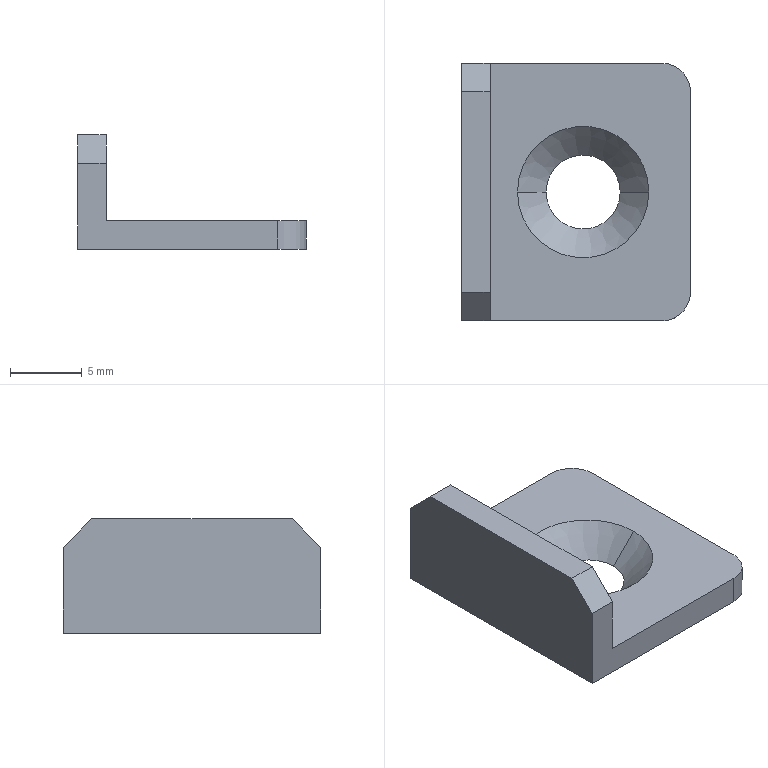Part | SolidWorks | features BaseBody 1 | 1 solid | 14 faces | box 16 x 18 x 8 mm | volume 697.494 mm3 | plane 10 | cone 2 | cylinder 2 | commonest cylinder face diameters 4 x2
STEP:
#1=CARTESIAN_POINT('',(-8.,-9.,4.));
#2=VERTEX_POINT('',#1);
#3=CARTESIAN_POINT('',(-8.,-7.,6.));
#4=VERTEX_POINT('',#3);
#5=CARTESIAN_POINT('',(-8.,-12.,1.));
#6=DIRECTION('',(0.,0.7071,0.7071));
#7=VECTOR('',#6,1000.);
#8=LINE('',#5,#7);
#9=EDGE_CURVE('',#2,#4,#8,.T.);
#10=ORIENTED_EDGE('',*,*,#9,.F.);
#11=CARTESIAN_POINT('',(-6.,-9.,4.));
#12=VERTEX_POINT('',#11);
#13=CARTESIAN_POINT('',(8.,-9.,4.));
#14=DIRECTION('',(-1.,0.,0.));
#15=VECTOR('',#14,1000.);
#16=LINE('',#13,#15);
#17=EDGE_CURVE('',#12,#2,#16,.T.);
#18=ORIENTED_EDGE('',*,*,#17,.F.);
#19=CARTESIAN_POINT('',(-6.,-7.,6.));
#20=VERTEX_POINT('',#19);
#21=CARTESIAN_POINT('',(-6.,-7.,6.));
#22=DIRECTION('',(0.,-0.7071,-0.7071));
#23=VECTOR('',#22,1000.);
#24=LINE('',#21,#23);
#25=EDGE_CURVE('',#20,#12,#24,.T.);
#26=ORIENTED_EDGE('',*,*,#25,.F.);
#27=CARTESIAN_POINT('',(0.,-7.,6.));
#28=DIRECTION('',(1.,0.,0.));
#29=VECTOR('',#28,1000.);
#30=LINE('',#27,#29);
#31=EDGE_CURVE('',#4,#20,#30,.T.);
#32=ORIENTED_EDGE('',*,*,#31,.F.);
#33=EDGE_LOOP('',(#10,#18,#26,#32));
#34=FACE_OUTER_BOUND('',#33,.T.);
#35=CARTESIAN_POINT('',(0.,-7.,6.));
#36=DIRECTION('',(0.,0.7071,-0.7071));
#37=DIRECTION('',(-1.,0.,0.));
#38=AXIS2_PLACEMENT_3D('',#35,#36,#37);
#39=PLANE('',#38);
#40=ADVANCED_FACE('',(#34),#39,.F.);
#41=CARTESIAN_POINT('',(-6.,9.,4.));
#42=VERTEX_POINT('',#41);
#43=CARTESIAN_POINT('',(-6.,7.,6.));
#44=VERTEX_POINT('',#43);
#45=CARTESIAN_POINT('',(-6.,7.,6.));
#46=DIRECTION('',(0.,-0.7071,0.7071));
#47=VECTOR('',#46,1000.);
#48=LINE('',#45,#47);
#49=EDGE_CURVE('',#42,#44,#48,.T.);
#50=ORIENTED_EDGE('',*,*,#49,.F.);
#51=CARTESIAN_POINT('',(-8.,9.,4.));
#52=VERTEX_POINT('',#51);
#53=CARTESIAN_POINT('',(8.,9.,4.));
#54=DIRECTION('',(1.,0.,0.));
#55=VECTOR('',#54,1000.);
#56=LINE('',#53,#55);
#57=EDGE_CURVE('',#52,#42,#56,.T.);
#58=ORIENTED_EDGE('',*,*,#57,.F.);
#59=CARTESIAN_POINT('',(-8.,7.,6.));
#60=VERTEX_POINT('',#59);
#61=CARTESIAN_POINT('',(-8.,3.,10.));
#62=DIRECTION('',(0.,0.7071,-0.7071));
#63=VECTOR('',#62,1000.);
#64=LINE('',#61,#63);
#65=EDGE_CURVE('',#60,#52,#64,.T.);
#66=ORIENTED_EDGE('',*,*,#65,.F.);
#67=CARTESIAN_POINT('',(0.,7.,6.));
#68=DIRECTION('',(-1.,0.,0.));
#69=VECTOR('',#68,1000.);
#70=LINE('',#67,#69);
#71=EDGE_CURVE('',#44,#60,#70,.T.);
#72=ORIENTED_EDGE('',*,*,#71,.F.);
#73=EDGE_LOOP('',(#50,#58,#66,#72));
#74=FACE_OUTER_BOUND('',#73,.T.);
#75=CARTESIAN_POINT('',(0.,7.,6.));
#76=DIRECTION('',(0.,-0.7071,-0.7071));
#77=DIRECTION('',(0.,0.7071,-0.7071));
#78=AXIS2_PLACEMENT_3D('',#75,#76,#77);
#79=PLANE('',#78);
#80=ADVANCED_FACE('',(#74),#79,.F.);
#81=CARTESIAN_POINT('',(-6.,9.,6.));
#82=DIRECTION('',(0.,1.,0.));
#83=VECTOR('',#82,1000.);
#84=LINE('',#81,#83);
#85=EDGE_CURVE('',#20,#44,#84,.T.);
#86=ORIENTED_EDGE('',*,*,#85,.T.);
#87=ORIENTED_EDGE('',*,*,#71,.T.);
#88=CARTESIAN_POINT('',(-8.,9.,6.));
#89=DIRECTION('',(0.,-1.,0.));
#90=VECTOR('',#89,1000.);
#91=LINE('',#88,#90);
#92=EDGE_CURVE('',#60,#4,#91,.T.);
#93=ORIENTED_EDGE('',*,*,#92,.T.);
#94=ORIENTED_EDGE('',*,*,#31,.T.);
#95=EDGE_LOOP('',(#86,#87,#93,#94));
#96=FACE_OUTER_BOUND('',#95,.T.);
#97=CARTESIAN_POINT('',(0.,0.,6.));
#98=DIRECTION('',(0.,0.,1.));
#99=DIRECTION('',(1.,0.,0.));
#100=AXIS2_PLACEMENT_3D('',#97,#98,#99);
#101=PLANE('',#100);
#102=ADVANCED_FACE('',(#96),#101,.T.);
#103=CARTESIAN_POINT('',(-6.,9.,0.));
#104=VERTEX_POINT('',#103);
#105=CARTESIAN_POINT('',(-6.,9.,6.));
#106=DIRECTION('',(0.,0.,-1.));
#107=VECTOR('',#106,1000.);
#108=LINE('',#105,#107);
#109=EDGE_CURVE('',#42,#104,#108,.T.);
#110=ORIENTED_EDGE('',*,*,#109,.F.);
#111=ORIENTED_EDGE('',*,*,#49,.T.);
#112=ORIENTED_EDGE('',*,*,#85,.F.);
#113=ORIENTED_EDGE('',*,*,#25,.T.);
#114=CARTESIAN_POINT('',(-6.,-9.,0.));
#115=VERTEX_POINT('',#114);
#116=CARTESIAN_POINT('',(-6.,-9.,6.));
#117=DIRECTION('',(0.,0.,-1.));
#118=VECTOR('',#117,1000.);
#119=LINE('',#116,#118);
#120=EDGE_CURVE('',#12,#115,#119,.T.);
#121=ORIENTED_EDGE('',*,*,#120,.T.);
#122=CARTESIAN_POINT('',(-6.,9.,0.));
#123=DIRECTION('',(0.,1.,0.));
#124=VECTOR('',#123,1000.);
#125=LINE('',#122,#124);
#126=EDGE_CURVE('',#115,#104,#125,.T.);
#127=ORIENTED_EDGE('',*,*,#126,.T.);
#128=EDGE_LOOP('',(#110,#111,#112,#113,#121,#127));
#129=FACE_OUTER_BOUND('',#128,.T.);
#130=CARTESIAN_POINT('',(-6.,9.,6.));
#131=DIRECTION('',(-1.,0.,0.));
#132=DIRECTION('',(0.,1.,0.));
#133=AXIS2_PLACEMENT_3D('',#130,#131,#132);
#134=PLANE('',#133);
#135=ADVANCED_FACE('',(#129),#134,.F.);
#136=CARTESIAN_POINT('',(-2.09,0.,-2.));
#137=VERTEX_POINT('',#136);
#138=CARTESIAN_POINT('',(-4.09,0.,0.));
#139=VERTEX_POINT('',#138);
#140=CARTESIAN_POINT('',(-4.09,0.,0.));
#141=DIRECTION('',(-0.7071,0.,0.7071));
#142=VECTOR('',#141,1000.);
#143=LINE('',#140,#142);
#144=EDGE_CURVE('',#137,#139,#143,.T.);
#145=ORIENTED_EDGE('',*,*,#144,.F.);
#146=CARTESIAN_POINT('',(3.09,0.,-2.));
#147=VERTEX_POINT('',#146);
#148=CARTESIAN_POINT('',(0.5,0.,-2.));
#149=DIRECTION('',(0.,0.,1.));
#150=DIRECTION('',(1.,0.,0.));
#151=AXIS2_PLACEMENT_3D('',#148,#149,#150);
#152=CIRCLE('',#151,2.59);
#153=EDGE_CURVE('',#147,#137,#152,.T.);
#154=ORIENTED_EDGE('',*,*,#153,.F.);
#155=CARTESIAN_POINT('',(5.09,0.,0.));
#156=VERTEX_POINT('',#155);
#157=CARTESIAN_POINT('',(5.09,0.,0.));
#158=DIRECTION('',(0.7071,0.,0.7071));
#159=VECTOR('',#158,1000.);
#160=LINE('',#157,#159);
#161=EDGE_CURVE('',#147,#156,#160,.T.);
#162=ORIENTED_EDGE('',*,*,#161,.T.);
#163=CARTESIAN_POINT('',(0.5,0.,0.));
#164=DIRECTION('',(0.,0.,1.));
#165=DIRECTION('',(1.,0.,0.));
#166=AXIS2_PLACEMENT_3D('',#163,#164,#165);
#167=CIRCLE('',#166,4.59);
#168=EDGE_CURVE('',#156,#139,#167,.T.);
#169=ORIENTED_EDGE('',*,*,#168,.T.);
#170=EDGE_LOOP('',(#145,#154,#162,#169));
#171=FACE_OUTER_BOUND('',#170,.T.);
#172=CARTESIAN_POINT('',(0.5,0.,0.));
#173=DIRECTION('',(0.,0.,1.));
#174=DIRECTION('',(1.,0.,0.));
#175=AXIS2_PLACEMENT_3D('',#172,#173,#174);
#176=CONICAL_SURFACE('',#175,4.59,0.7854);
#177=ADVANCED_FACE('',(#171),#176,.F.);
#178=CARTESIAN_POINT('',(8.,-7.,-2.));
#179=VERTEX_POINT('',#178);
#180=CARTESIAN_POINT('',(6.,-9.,-2.));
#181=VERTEX_POINT('',#180);
#182=CARTESIAN_POINT('',(6.,-7.,-2.));
#183=DIRECTION('',(0.,0.,-1.));
#184=DIRECTION('',(1.,0.,0.));
#185=AXIS2_PLACEMENT_3D('',#182,#183,#184);
#186=CIRCLE('',#185,2.);
#187=EDGE_CURVE('',#179,#181,#186,.T.);
#188=ORIENTED_EDGE('',*,*,#187,.F.);
#189=CARTESIAN_POINT('',(8.,-7.,0.));
#190=VERTEX_POINT('',#189);
#191=CARTESIAN_POINT('',(8.,-7.,-2.));
#192=DIRECTION('',(0.,0.,-1.));
#193=VECTOR('',#192,1000.);
#194=LINE('',#191,#193);
#195=EDGE_CURVE('',#190,#179,#194,.T.);
#196=ORIENTED_EDGE('',*,*,#195,.F.);
#197=CARTESIAN_POINT('',(6.,-9.,0.));
#198=VERTEX_POINT('',#197);
#199=CARTESIAN_POINT('',(6.,-7.,0.));
#200=DIRECTION('',(0.,0.,1.));
#201=DIRECTION('',(1.,0.,0.));
#202=AXIS2_PLACEMENT_3D('',#199,#200,#201);
#203=CIRCLE('',#202,2.);
#204=EDGE_CURVE('',#198,#190,#203,.T.);
#205=ORIENTED_EDGE('',*,*,#204,.F.);
#206=CARTESIAN_POINT('',(6.,-9.,-2.));
#207=DIRECTION('',(0.,0.,1.));
#208=VECTOR('',#207,1000.);
#209=LINE('',#206,#208);
#210=EDGE_CURVE('',#181,#198,#209,.T.);
#211=ORIENTED_EDGE('',*,*,#210,.F.);
#212=EDGE_LOOP('',(#188,#196,#205,#211));
#213=FACE_OUTER_BOUND('',#212,.T.);
#214=CARTESIAN_POINT('',(6.,-7.,-2.));
#215=DIRECTION('',(0.,0.,1.));
#216=DIRECTION('',(1.,0.,0.));
#217=AXIS2_PLACEMENT_3D('',#214,#215,#216);
#218=CYLINDRICAL_SURFACE('',#217,2.);
#219=ADVANCED_FACE('',(#213),#218,.T.);
#220=CARTESIAN_POINT('',(6.,9.,-2.));
#221=VERTEX_POINT('',#220);
#222=CARTESIAN_POINT('',(8.,7.,-2.));
#223=VERTEX_POINT('',#222);
#224=CARTESIAN_POINT('',(6.,7.,-2.));
#225=DIRECTION('',(0.,0.,-1.));
#226=DIRECTION('',(1.,0.,0.));
#227=AXIS2_PLACEMENT_3D('',#224,#225,#226);
#228=CIRCLE('',#227,2.);
#229=EDGE_CURVE('',#221,#223,#228,.T.);
#230=ORIENTED_EDGE('',*,*,#229,.F.);
#231=CARTESIAN_POINT('',(6.,9.,0.));
#232=VERTEX_POINT('',#231);
#233=CARTESIAN_POINT('',(6.,9.,-2.));
#234=DIRECTION('',(0.,0.,-1.));
#235=VECTOR('',#234,1000.);
#236=LINE('',#233,#235);
#237=EDGE_CURVE('',#232,#221,#236,.T.);
#238=ORIENTED_EDGE('',*,*,#237,.F.);
#239=CARTESIAN_POINT('',(8.,7.,0.));
#240=VERTEX_POINT('',#239);
#241=CARTESIAN_POINT('',(6.,7.,0.));
#242=DIRECTION('',(0.,0.,1.));
#243=DIRECTION('',(1.,0.,0.));
#244=AXIS2_PLACEMENT_3D('',#241,#242,#243);
#245=CIRCLE('',#244,2.);
#246=EDGE_CURVE('',#240,#232,#245,.T.);
#247=ORIENTED_EDGE('',*,*,#246,.F.);
#248=CARTESIAN_POINT('',(8.,7.,-2.));
#249=DIRECTION('',(0.,0.,1.));
#250=VECTOR('',#249,1000.);
#251=LINE('',#248,#250);
#252=EDGE_CURVE('',#223,#240,#251,.T.);
#253=ORIENTED_EDGE('',*,*,#252,.F.);
#254=EDGE_LOOP('',(#230,#238,#247,#253));
#255=FACE_OUTER_BOUND('',#254,.T.);
#256=CARTESIAN_POINT('',(6.,7.,-2.));
#257=DIRECTION('',(0.,0.,1.));
#258=DIRECTION('',(1.,0.,0.));
#259=AXIS2_PLACEMENT_3D('',#256,#257,#258);
#260=CYLINDRICAL_SURFACE('',#259,2.);
#261=ADVANCED_FACE('',(#255),#260,.T.);
#262=ORIENTED_EDGE('',*,*,#168,.F.);
#263=CARTESIAN_POINT('',(0.5,0.,0.));
#264=DIRECTION('',(0.,0.,1.));
#265=DIRECTION('',(1.,0.,0.));
#266=AXIS2_PLACEMENT_3D('',#263,#264,#265);
#267=CIRCLE('',#266,4.59);
#268=EDGE_CURVE('',#139,#156,#267,.T.);
#269=ORIENTED_EDGE('',*,*,#268,.F.);
#270=EDGE_LOOP('',(#262,#269));
#271=FACE_BOUND('',#270,.T.);
#272=ORIENTED_EDGE('',*,*,#126,.F.);
#273=CARTESIAN_POINT('',(8.,-9.,0.));
#274=DIRECTION('',(1.,0.,0.));
#275=VECTOR('',#274,1000.);
#276=LINE('',#273,#275);
#277=EDGE_CURVE('',#115,#198,#276,.T.);
#278=ORIENTED_EDGE('',*,*,#277,.T.);
#279=ORIENTED_EDGE('',*,*,#204,.T.);
#280=CARTESIAN_POINT('',(8.,-9.,0.));
#281=DIRECTION('',(0.,1.,0.));
#282=VECTOR('',#281,1000.);
#283=LINE('',#280,#282);
#284=EDGE_CURVE('',#190,#240,#283,.T.);
#285=ORIENTED_EDGE('',*,*,#284,.T.);
#286=ORIENTED_EDGE('',*,*,#246,.T.);
#287=CARTESIAN_POINT('',(8.,9.,0.));
#288=DIRECTION('',(-1.,0.,0.));
#289=VECTOR('',#288,1000.);
#290=LINE('',#287,#289);
#291=EDGE_CURVE('',#232,#104,#290,.T.);
#292=ORIENTED_EDGE('',*,*,#291,.T.);
#293=EDGE_LOOP('',(#272,#278,#279,#285,#286,#292));
#294=FACE_OUTER_BOUND('',#293,.T.);
#295=CARTESIAN_POINT('',(0.,0.,0.));
#296=DIRECTION('',(0.,0.,1.));
#297=DIRECTION('',(1.,0.,0.));
#298=AXIS2_PLACEMENT_3D('',#295,#296,#297);
#299=PLANE('',#298);
#300=ADVANCED_FACE('',(#271,#294),#299,.T.);
#301=ORIENTED_EDGE('',*,*,#153,.T.);
#302=CARTESIAN_POINT('',(0.5,0.,-2.));
#303=DIRECTION('',(0.,0.,1.));
#304=DIRECTION('',(1.,0.,0.));
#305=AXIS2_PLACEMENT_3D('',#302,#303,#304);
#306=CIRCLE('',#305,2.59);
#307=EDGE_CURVE('',#137,#147,#306,.T.);
#308=ORIENTED_EDGE('',*,*,#307,.T.);
#309=EDGE_LOOP('',(#301,#308));
#310=FACE_BOUND('',#309,.T.);
#311=CARTESIAN_POINT('',(-8.,9.,-2.));
#312=VERTEX_POINT('',#311);
#313=CARTESIAN_POINT('',(8.,9.,-2.));
#314=DIRECTION('',(-1.,0.,0.));
#315=VECTOR('',#314,1000.);
#316=LINE('',#313,#315);
#317=EDGE_CURVE('',#221,#312,#316,.T.);
#318=ORIENTED_EDGE('',*,*,#317,.F.);
#319=ORIENTED_EDGE('',*,*,#229,.T.);
#320=CARTESIAN_POINT('',(8.,-9.,-2.));
#321=DIRECTION('',(0.,1.,0.));
#322=VECTOR('',#321,1000.);
#323=LINE('',#320,#322);
#324=EDGE_CURVE('',#179,#223,#323,.T.);
#325=ORIENTED_EDGE('',*,*,#324,.F.);
#326=ORIENTED_EDGE('',*,*,#187,.T.);
#327=CARTESIAN_POINT('',(-8.,-9.,-2.));
#328=VERTEX_POINT('',#327);
#329=CARTESIAN_POINT('',(8.,-9.,-2.));
#330=DIRECTION('',(1.,0.,0.));
#331=VECTOR('',#330,1000.);
#332=LINE('',#329,#331);
#333=EDGE_CURVE('',#328,#181,#332,.T.);
#334=ORIENTED_EDGE('',*,*,#333,.F.);
#335=CARTESIAN_POINT('',(-8.,-9.,-2.));
#336=DIRECTION('',(0.,-1.,0.));
#337=VECTOR('',#336,1000.);
#338=LINE('',#335,#337);
#339=EDGE_CURVE('',#312,#328,#338,.T.);
#340=ORIENTED_EDGE('',*,*,#339,.F.);
#341=EDGE_LOOP('',(#318,#319,#325,#326,#334,#340));
#342=FACE_OUTER_BOUND('',#341,.T.);
#343=CARTESIAN_POINT('',(0.,0.,-2.));
#344=DIRECTION('',(0.,0.,1.));
#345=DIRECTION('',(1.,0.,0.));
#346=AXIS2_PLACEMENT_3D('',#343,#344,#345);
#347=PLANE('',#346);
#348=ADVANCED_FACE('',(#310,#342),#347,.F.);
#349=ORIENTED_EDGE('',*,*,#120,.F.);
#350=ORIENTED_EDGE('',*,*,#17,.T.);
#351=CARTESIAN_POINT('',(-8.,-9.,-2.));
#352=DIRECTION('',(0.,0.,1.));
#353=VECTOR('',#352,1000.);
#354=LINE('',#351,#353);
#355=EDGE_CURVE('',#328,#2,#354,.T.);
#356=ORIENTED_EDGE('',*,*,#355,.F.);
#357=ORIENTED_EDGE('',*,*,#333,.T.);
#358=ORIENTED_EDGE('',*,*,#210,.T.);
#359=ORIENTED_EDGE('',*,*,#277,.F.);
#360=EDGE_LOOP('',(#349,#350,#356,#357,#358,#359));
#361=FACE_OUTER_BOUND('',#360,.T.);
#362=CARTESIAN_POINT('',(8.,-9.,-2.));
#363=DIRECTION('',(0.,-1.,0.));
#364=DIRECTION('',(0.,0.,-1.));
#365=AXIS2_PLACEMENT_3D('',#362,#363,#364);
#366=PLANE('',#365);
#367=ADVANCED_FACE('',(#361),#366,.T.);
#368=ORIENTED_EDGE('',*,*,#324,.T.);
#369=ORIENTED_EDGE('',*,*,#252,.T.);
#370=ORIENTED_EDGE('',*,*,#284,.F.);
#371=ORIENTED_EDGE('',*,*,#195,.T.);
#372=EDGE_LOOP('',(#368,#369,#370,#371));
#373=FACE_OUTER_BOUND('',#372,.T.);
#374=CARTESIAN_POINT('',(8.,-9.,-2.));
#375=DIRECTION('',(1.,0.,0.));
#376=DIRECTION('',(0.,1.,0.));
#377=AXIS2_PLACEMENT_3D('',#374,#375,#376);
#378=PLANE('',#377);
#379=ADVANCED_FACE('',(#373),#378,.T.);
#380=CARTESIAN_POINT('',(-8.,9.,-2.));
#381=DIRECTION('',(0.,0.,1.));
#382=VECTOR('',#381,1000.);
#383=LINE('',#380,#382);
#384=EDGE_CURVE('',#312,#52,#383,.T.);
#385=ORIENTED_EDGE('',*,*,#384,.T.);
#386=ORIENTED_EDGE('',*,*,#57,.T.);
#387=ORIENTED_EDGE('',*,*,#109,.T.);
#388=ORIENTED_EDGE('',*,*,#291,.F.);
#389=ORIENTED_EDGE('',*,*,#237,.T.);
#390=ORIENTED_EDGE('',*,*,#317,.T.);
#391=EDGE_LOOP('',(#385,#386,#387,#388,#389,#390));
#392=FACE_OUTER_BOUND('',#391,.T.);
#393=CARTESIAN_POINT('',(8.,9.,-2.));
#394=DIRECTION('',(0.,1.,0.));
#395=DIRECTION('',(1.,0.,0.));
#396=AXIS2_PLACEMENT_3D('',#393,#394,#395);
#397=PLANE('',#396);
#398=ADVANCED_FACE('',(#392),#397,.T.);
#399=ORIENTED_EDGE('',*,*,#92,.F.);
#400=ORIENTED_EDGE('',*,*,#65,.T.);
#401=ORIENTED_EDGE('',*,*,#384,.F.);
#402=ORIENTED_EDGE('',*,*,#339,.T.);
#403=ORIENTED_EDGE('',*,*,#355,.T.);
#404=ORIENTED_EDGE('',*,*,#9,.T.);
#405=EDGE_LOOP('',(#399,#400,#401,#402,#403,#404));
#406=FACE_OUTER_BOUND('',#405,.T.);
#407=CARTESIAN_POINT('',(-8.,-9.,-2.));
#408=DIRECTION('',(-1.,0.,0.));
#409=DIRECTION('',(0.,0.,1.));
#410=AXIS2_PLACEMENT_3D('',#407,#408,#409);
#411=PLANE('',#410);
#412=ADVANCED_FACE('',(#406),#411,.T.);
#413=ORIENTED_EDGE('',*,*,#307,.F.);
#414=ORIENTED_EDGE('',*,*,#144,.T.);
#415=ORIENTED_EDGE('',*,*,#268,.T.);
#416=ORIENTED_EDGE('',*,*,#161,.F.);
#417=EDGE_LOOP('',(#413,#414,#415,#416));
#418=FACE_OUTER_BOUND('',#417,.T.);
#419=CARTESIAN_POINT('',(0.5,0.,0.));
#420=DIRECTION('',(0.,0.,1.));
#421=DIRECTION('',(1.,0.,0.));
#422=AXIS2_PLACEMENT_3D('',#419,#420,#421);
#423=CONICAL_SURFACE('',#422,4.59,0.7854);
#424=ADVANCED_FACE('',(#418),#423,.F.);
#425=CLOSED_SHELL('',(#40,#80,#102,#135,#177,#219,#261,#300,#348,#367,#379,#398,#412,#424));
#426=MANIFOLD_SOLID_BREP('',#425);
#427=CARTESIAN_POINT('',(0.,0.,0.));
#428=DIRECTION('',(0.,0.,1.));
#429=DIRECTION('',(1.,0.,0.));
#430=AXIS2_PLACEMENT_3D('',#427,#428,#429);
#431=(LENGTH_UNIT()NAMED_UNIT(*)SI_UNIT(.MILLI.,.METRE.));
#432=UNCERTAINTY_MEASURE_WITH_UNIT(LENGTH_MEASURE(0.00001),#431,'','');
#433=(NAMED_UNIT(*)PLANE_ANGLE_UNIT()SI_UNIT($,.RADIAN.));
#434=(NAMED_UNIT(*)SI_UNIT($,.STERADIAN.)SOLID_ANGLE_UNIT());
#435=(GEOMETRIC_REPRESENTATION_CONTEXT(3)GLOBAL_UNCERTAINTY_ASSIGNED_CONTEXT((#432))GLOBAL_UNIT_ASSIGNED_CONTEXT((#431,#433,#434))REPRESENTATION_CONTEXT('',''));
#436=ADVANCED_BREP_SHAPE_REPRESENTATION('',(#426,#430),#435);